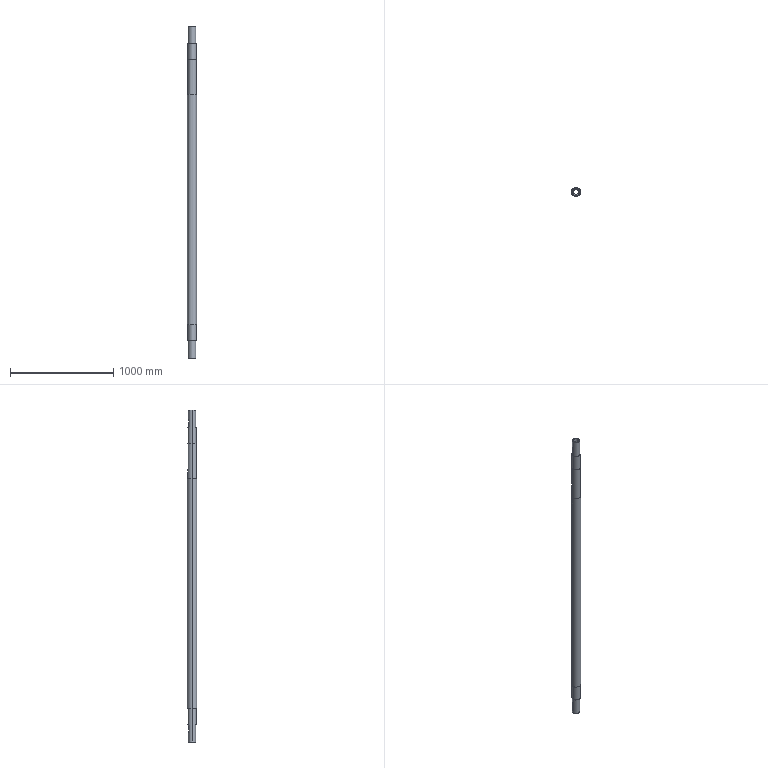Part | SolidWorks | features ICE 9, MirrorPattern 2, Chamfer 1, Extrusion 1 | 1 solid | 39 faces | box 89 x 89 x 3215 mm | volume 11535395 mm3 | cylinder 23 | plane 16 | commonest cylinder face diameters 20 x6 70 x4 80 x4 22 x3 53 x2 85 x2
STEP:
#1=CARTESIAN_POINT('',(0.,33.5,2636.));
#2=VERTEX_POINT('',#1);
#3=CARTESIAN_POINT('',(11.,33.5,2625.));
#4=VERTEX_POINT('',#3);
#5=CARTESIAN_POINT('',(0.,33.5,2625.));
#6=DIRECTION('',(0.,1.,0.));
#7=DIRECTION('',(0.,0.,1.));
#8=AXIS2_PLACEMENT_3D('',#5,#6,#7);
#9=CIRCLE('',#8,11.);
#10=EDGE_CURVE('',#2,#4,#9,.T.);
#11=ORIENTED_EDGE('',*,*,#10,.F.);
#12=CARTESIAN_POINT('',(0.,42.5,2636.));
#13=VERTEX_POINT('',#12);
#14=CARTESIAN_POINT('',(0.,33.5,2636.));
#15=DIRECTION('',(0.,1.,0.));
#16=VECTOR('',#15,1000.);
#17=LINE('',#14,#16);
#18=EDGE_CURVE('',#2,#13,#17,.T.);
#19=ORIENTED_EDGE('',*,*,#18,.T.);
#20=CARTESIAN_POINT('',(11.,41.052,2625.));
#21=VERTEX_POINT('',#20);
#22=CARTESIAN_POINT('',(0.,42.5,2636.));
#23=CARTESIAN_POINT('',(0.7204,42.5,2636.));
#24=CARTESIAN_POINT('',(1.452,42.481,2635.927));
#25=CARTESIAN_POINT('',(2.864,42.409,2635.645));
#26=CARTESIAN_POINT('',(3.551,42.357,2635.436));
#27=CARTESIAN_POINT('',(4.552,42.257,2635.02));
#28=CARTESIAN_POINT('',(4.881,42.22,2634.864));
#29=CARTESIAN_POINT('',(5.514,42.142,2634.525));
#30=CARTESIAN_POINT('',(5.821,42.101,2634.341));
#31=CARTESIAN_POINT('',(6.414,42.014,2633.943));
#32=CARTESIAN_POINT('',(6.701,41.969,2633.73));
#33=CARTESIAN_POINT('',(7.256,41.877,2633.276));
#34=CARTESIAN_POINT('',(7.524,41.829,2633.032));
#35=CARTESIAN_POINT('',(8.287,41.687,2632.269));
#36=CARTESIAN_POINT('',(8.74,41.594,2631.717));
#37=CARTESIAN_POINT('',(9.337,41.462,2630.827));
#38=CARTESIAN_POINT('',(9.522,41.42,2630.519));
#39=CARTESIAN_POINT('',(9.864,41.34,2629.882));
#40=CARTESIAN_POINT('',(10.019,41.302,2629.555));
#41=CARTESIAN_POINT('',(10.433,41.201,2628.56));
#42=CARTESIAN_POINT('',(10.642,41.146,2627.875));
#43=CARTESIAN_POINT('',(10.855,41.09,2626.814));
#44=CARTESIAN_POINT('',(10.91,41.076,2626.452));
#45=CARTESIAN_POINT('',(10.982,41.057,2625.728));
#46=CARTESIAN_POINT('',(11.,41.052,2625.365));
#47=CARTESIAN_POINT('',(11.,41.052,2625.));
#48=B_SPLINE_CURVE_WITH_KNOTS('',3,(#22,#23,#24,#25,#26,#27,#28,#29,#30,#31,#32,#33,#34,#35,#36,#37,#38,#39,#40,#41,#42,#43,#44,#45,#46,#47),.UNSPECIFIED.,.F.,.F.,(4,2,2,2,2,2,2,2,2,2,2,2,4),(0.01727,0.01943,0.02159,0.02267,0.02374,0.02482,0.0259,0.02806,0.02914,0.03021,0.03237,0.03345,0.03453),.UNSPECIFIED.);
#49=EDGE_CURVE('',#13,#21,#48,.T.);
#50=ORIENTED_EDGE('',*,*,#49,.T.);
#51=CARTESIAN_POINT('',(11.,33.5,2625.));
#52=DIRECTION('',(0.,1.,0.));
#53=VECTOR('',#52,1000.);
#54=LINE('',#51,#53);
#55=EDGE_CURVE('',#4,#21,#54,.T.);
#56=ORIENTED_EDGE('',*,*,#55,.F.);
#57=EDGE_LOOP('',(#11,#19,#50,#56));
#58=FACE_OUTER_BOUND('',#57,.T.);
#59=CARTESIAN_POINT('',(0.,33.5,2625.));
#60=DIRECTION('',(0.,1.,0.));
#61=DIRECTION('',(0.,0.,1.));
#62=AXIS2_PLACEMENT_3D('',#59,#60,#61);
#63=CYLINDRICAL_SURFACE('',#62,11.);
#64=ADVANCED_FACE('',(#58),#63,.F.);
#65=CARTESIAN_POINT('',(10.,27.5,150.));
#66=VERTEX_POINT('',#65);
#67=CARTESIAN_POINT('',(0.,27.5,160.));
#68=VERTEX_POINT('',#67);
#69=CARTESIAN_POINT('',(0.,27.5,150.));
#70=DIRECTION('',(0.,-1.,0.));
#71=DIRECTION('',(0.,0.,-1.));
#72=AXIS2_PLACEMENT_3D('',#69,#70,#71);
#73=CIRCLE('',#72,10.);
#74=EDGE_CURVE('',#66,#68,#73,.T.);
#75=ORIENTED_EDGE('',*,*,#74,.T.);
#76=CARTESIAN_POINT('',(0.,35.,160.));
#77=VERTEX_POINT('',#76);
#78=CARTESIAN_POINT('',(0.,27.5,160.));
#79=DIRECTION('',(0.,1.,0.));
#80=VECTOR('',#79,1000.);
#81=LINE('',#78,#80);
#82=EDGE_CURVE('',#68,#77,#81,.T.);
#83=ORIENTED_EDGE('',*,*,#82,.T.);
#84=CARTESIAN_POINT('',(10.,33.541,150.));
#85=VERTEX_POINT('',#84);
#86=CARTESIAN_POINT('',(0.,35.,160.));
#87=CARTESIAN_POINT('',(0.6556,35.,160.));
#88=CARTESIAN_POINT('',(1.322,34.981,159.934));
#89=CARTESIAN_POINT('',(2.606,34.909,159.677));
#90=CARTESIAN_POINT('',(3.23,34.856,159.487));
#91=CARTESIAN_POINT('',(4.141,34.756,159.108));
#92=CARTESIAN_POINT('',(4.439,34.719,158.966));
#93=CARTESIAN_POINT('',(5.015,34.64,158.658));
#94=CARTESIAN_POINT('',(5.293,34.598,158.49));
#95=CARTESIAN_POINT('',(5.833,34.512,158.129));
#96=CARTESIAN_POINT('',(6.093,34.466,157.936));
#97=CARTESIAN_POINT('',(6.597,34.374,157.522));
#98=CARTESIAN_POINT('',(6.841,34.326,157.301));
#99=CARTESIAN_POINT('',(7.534,34.183,156.608));
#100=CARTESIAN_POINT('',(7.945,34.088,156.108));
#101=CARTESIAN_POINT('',(8.668,33.912,155.029));
#102=CARTESIAN_POINT('',(8.982,33.829,154.444));
#103=CARTESIAN_POINT('',(9.483,33.692,153.24));
#104=CARTESIAN_POINT('',(9.674,33.637,152.617));
#105=CARTESIAN_POINT('',(9.868,33.58,151.65));
#106=CARTESIAN_POINT('',(9.918,33.565,151.321));
#107=CARTESIAN_POINT('',(9.984,33.546,150.663));
#108=CARTESIAN_POINT('',(10.,33.541,150.332));
#109=CARTESIAN_POINT('',(10.,33.541,150.));
#110=B_SPLINE_CURVE_WITH_KNOTS('',3,(#86,#87,#88,#89,#90,#91,#92,#93,#94,#95,#96,#97,#98,#99,#100,#101,#102,#103,#104,#105,#106,#107,#108,#109),.UNSPECIFIED.,.F.,.F.,(4,2,2,2,2,2,2,2,2,2,2,4),(0.01572,0.01768,0.01964,0.02062,0.02161,0.02259,0.02357,0.02553,0.02749,0.02946,0.03044,0.03142),.UNSPECIFIED.);
#111=EDGE_CURVE('',#77,#85,#110,.T.);
#112=ORIENTED_EDGE('',*,*,#111,.T.);
#113=CARTESIAN_POINT('',(10.,27.5,150.));
#114=DIRECTION('',(0.,1.,0.));
#115=VECTOR('',#114,1000.);
#116=LINE('',#113,#115);
#117=EDGE_CURVE('',#66,#85,#116,.T.);
#118=ORIENTED_EDGE('',*,*,#117,.F.);
#119=EDGE_LOOP('',(#75,#83,#112,#118));
#120=FACE_OUTER_BOUND('',#119,.T.);
#121=CARTESIAN_POINT('',(0.,27.5,150.));
#122=DIRECTION('',(0.,1.,0.));
#123=DIRECTION('',(0.,0.,1.));
#124=AXIS2_PLACEMENT_3D('',#121,#122,#123);
#125=CYLINDRICAL_SURFACE('',#124,10.);
#126=ADVANCED_FACE('',(#120),#125,.F.);
#127=CARTESIAN_POINT('',(0.,27.5,3130.));
#128=VERTEX_POINT('',#127);
#129=CARTESIAN_POINT('',(10.,27.5,3120.));
#130=VERTEX_POINT('',#129);
#131=CARTESIAN_POINT('',(0.,27.5,3120.));
#132=DIRECTION('',(0.,1.,0.));
#133=DIRECTION('',(0.,0.,1.));
#134=AXIS2_PLACEMENT_3D('',#131,#132,#133);
#135=CIRCLE('',#134,10.);
#136=EDGE_CURVE('',#128,#130,#135,.T.);
#137=ORIENTED_EDGE('',*,*,#136,.F.);
#138=CARTESIAN_POINT('',(0.,35.,3130.));
#139=VERTEX_POINT('',#138);
#140=CARTESIAN_POINT('',(0.,27.5,3130.));
#141=DIRECTION('',(0.,1.,0.));
#142=VECTOR('',#141,1000.);
#143=LINE('',#140,#142);
#144=EDGE_CURVE('',#128,#139,#143,.T.);
#145=ORIENTED_EDGE('',*,*,#144,.T.);
#146=CARTESIAN_POINT('',(10.,33.541,3120.));
#147=VERTEX_POINT('',#146);
#148=CARTESIAN_POINT('',(0.,35.,3130.));
#149=CARTESIAN_POINT('',(0.6556,35.,3130.));
#150=CARTESIAN_POINT('',(1.322,34.981,3129.934));
#151=CARTESIAN_POINT('',(2.606,34.909,3129.677));
#152=CARTESIAN_POINT('',(3.23,34.856,3129.487));
#153=CARTESIAN_POINT('',(4.141,34.756,3129.108));
#154=CARTESIAN_POINT('',(4.439,34.719,3128.966));
#155=CARTESIAN_POINT('',(5.015,34.64,3128.658));
#156=CARTESIAN_POINT('',(5.293,34.598,3128.49));
#157=CARTESIAN_POINT('',(5.833,34.512,3128.129));
#158=CARTESIAN_POINT('',(6.093,34.466,3127.936));
#159=CARTESIAN_POINT('',(6.597,34.374,3127.522));
#160=CARTESIAN_POINT('',(6.841,34.326,3127.301));
#161=CARTESIAN_POINT('',(7.534,34.183,3126.608));
#162=CARTESIAN_POINT('',(7.945,34.088,3126.108));
#163=CARTESIAN_POINT('',(8.668,33.912,3125.029));
#164=CARTESIAN_POINT('',(8.982,33.829,3124.444));
#165=CARTESIAN_POINT('',(9.483,33.692,3123.24));
#166=CARTESIAN_POINT('',(9.674,33.637,3122.617));
#167=CARTESIAN_POINT('',(9.868,33.58,3121.65));
#168=CARTESIAN_POINT('',(9.918,33.565,3121.321));
#169=CARTESIAN_POINT('',(9.984,33.546,3120.663));
#170=CARTESIAN_POINT('',(10.,33.541,3120.332));
#171=CARTESIAN_POINT('',(10.,33.541,3120.));
#172=B_SPLINE_CURVE_WITH_KNOTS('',3,(#148,#149,#150,#151,#152,#153,#154,#155,#156,#157,#158,#159,#160,#161,#162,#163,#164,#165,#166,#167,#168,#169,#170,#171),.UNSPECIFIED.,.F.,.F.,(4,2,2,2,2,2,2,2,2,2,2,4),(0.01572,0.01768,0.01964,0.02062,0.02161,0.02259,0.02357,0.02553,0.02749,0.02946,0.03044,0.03142),.UNSPECIFIED.);
#173=EDGE_CURVE('',#139,#147,#172,.T.);
#174=ORIENTED_EDGE('',*,*,#173,.T.);
#175=CARTESIAN_POINT('',(10.,27.5,3120.));
#176=DIRECTION('',(0.,1.,0.));
#177=VECTOR('',#176,1000.);
#178=LINE('',#175,#177);
#179=EDGE_CURVE('',#130,#147,#178,.T.);
#180=ORIENTED_EDGE('',*,*,#179,.F.);
#181=EDGE_LOOP('',(#137,#145,#174,#180));
#182=FACE_OUTER_BOUND('',#181,.T.);
#183=CARTESIAN_POINT('',(0.,27.5,3120.));
#184=DIRECTION('',(0.,1.,0.));
#185=DIRECTION('',(0.,0.,1.));
#186=AXIS2_PLACEMENT_3D('',#183,#184,#185);
#187=CYLINDRICAL_SURFACE('',#186,10.);
#188=ADVANCED_FACE('',(#182),#187,.F.);
#189=CARTESIAN_POINT('',(40.,0.,320.));
#190=VERTEX_POINT('',#189);
#191=CARTESIAN_POINT('',(-40.,0.,320.));
#192=VERTEX_POINT('',#191);
#193=CARTESIAN_POINT('',(0.,0.,320.));
#194=DIRECTION('',(0.,0.,1.));
#195=DIRECTION('',(1.,0.,0.));
#196=AXIS2_PLACEMENT_3D('',#193,#194,#195);
#197=CIRCLE('',#196,40.);
#198=EDGE_CURVE('',#190,#192,#197,.T.);
#199=ORIENTED_EDGE('',*,*,#198,.F.);
#200=CARTESIAN_POINT('',(40.,0.,165.));
#201=VERTEX_POINT('',#200);
#202=CARTESIAN_POINT('',(40.,0.,320.));
#203=DIRECTION('',(0.,0.,-1.));
#204=VECTOR('',#203,1000.);
#205=LINE('',#202,#204);
#206=EDGE_CURVE('',#190,#201,#205,.T.);
#207=ORIENTED_EDGE('',*,*,#206,.T.);
#208=CARTESIAN_POINT('',(-40.,0.,165.));
#209=VERTEX_POINT('',#208);
#210=CARTESIAN_POINT('',(0.,0.,165.));
#211=DIRECTION('',(0.,0.,1.));
#212=DIRECTION('',(1.,0.,0.));
#213=AXIS2_PLACEMENT_3D('',#210,#211,#212);
#214=CIRCLE('',#213,40.);
#215=EDGE_CURVE('',#201,#209,#214,.T.);
#216=ORIENTED_EDGE('',*,*,#215,.T.);
#217=CARTESIAN_POINT('',(-40.,0.,320.));
#218=DIRECTION('',(0.,0.,-1.));
#219=VECTOR('',#218,1000.);
#220=LINE('',#217,#219);
#221=EDGE_CURVE('',#192,#209,#220,.T.);
#222=ORIENTED_EDGE('',*,*,#221,.F.);
#223=EDGE_LOOP('',(#199,#207,#216,#222));
#224=FACE_OUTER_BOUND('',#223,.T.);
#225=CARTESIAN_POINT('',(0.,0.,320.));
#226=DIRECTION('',(0.,0.,-1.));
#227=DIRECTION('',(-1.,0.,0.));
#228=AXIS2_PLACEMENT_3D('',#225,#226,#227);
#229=CYLINDRICAL_SURFACE('',#228,40.);
#230=ADVANCED_FACE('',(#224),#229,.T.);
#231=CARTESIAN_POINT('',(-10.,33.541,3120.));
#232=VERTEX_POINT('',#231);
#233=CARTESIAN_POINT('',(-10.,33.541,3120.));
#234=CARTESIAN_POINT('',(-10.,33.541,3120.665));
#235=CARTESIAN_POINT('',(-9.934,33.561,3121.317));
#236=CARTESIAN_POINT('',(-9.742,33.617,3122.28));
#237=CARTESIAN_POINT('',(-9.662,33.64,3122.598));
#238=CARTESIAN_POINT('',(-9.47,33.695,3123.228));
#239=CARTESIAN_POINT('',(-9.358,33.726,3123.54));
#240=CARTESIAN_POINT('',(-8.981,33.829,3124.447));
#241=CARTESIAN_POINT('',(-8.673,33.91,3125.02));
#242=CARTESIAN_POINT('',(-8.129,34.044,3125.834));
#243=CARTESIAN_POINT('',(-7.932,34.09,3126.099));
#244=CARTESIAN_POINT('',(-7.516,34.184,3126.604));
#245=CARTESIAN_POINT('',(-7.298,34.232,3126.845));
#246=CARTESIAN_POINT('',(-6.609,34.374,3127.533));
#247=CARTESIAN_POINT('',(-6.108,34.467,3127.945));
#248=CARTESIAN_POINT('',(-5.015,34.643,3128.677));
#249=CARTESIAN_POINT('',(-4.438,34.723,3128.985));
#250=CARTESIAN_POINT('',(-3.536,34.822,3129.36));
#251=CARTESIAN_POINT('',(-3.229,34.852,3129.47));
#252=CARTESIAN_POINT('',(-2.6,34.905,3129.662));
#253=CARTESIAN_POINT('',(-2.278,34.927,3129.743));
#254=CARTESIAN_POINT('',(-1.308,34.982,3129.936));
#255=CARTESIAN_POINT('',(-0.6564,35.,3130.));
#256=CARTESIAN_POINT('',(0.,35.,3130.));
#257=B_SPLINE_CURVE_WITH_KNOTS('',3,(#233,#234,#235,#236,#237,#238,#239,#240,#241,#242,#243,#244,#245,#246,#247,#248,#249,#250,#251,#252,#253,#254,#255,#256),.UNSPECIFIED.,.F.,.F.,(4,2,2,2,2,2,2,2,2,2,2,4),(0.,0.001965,0.002947,0.00393,0.005894,0.006877,0.007859,0.009824,0.01179,0.01277,0.01375,0.01572),.UNSPECIFIED.);
#258=EDGE_CURVE('',#232,#139,#257,.T.);
#259=ORIENTED_EDGE('',*,*,#258,.F.);
#260=CARTESIAN_POINT('',(-10.,33.541,3065.));
#261=VERTEX_POINT('',#260);
#262=CARTESIAN_POINT('',(-10.,33.541,2943.934));
#263=DIRECTION('',(0.,0.,1.));
#264=VECTOR('',#263,1000.);
#265=LINE('',#262,#264);
#266=EDGE_CURVE('',#261,#232,#265,.T.);
#267=ORIENTED_EDGE('',*,*,#266,.F.);
#268=CARTESIAN_POINT('',(10.,33.541,3065.));
#269=VERTEX_POINT('',#268);
#270=CARTESIAN_POINT('',(10.,33.541,3065.));
#271=CARTESIAN_POINT('',(10.,33.541,3064.336));
#272=CARTESIAN_POINT('',(9.934,33.561,3063.683));
#273=CARTESIAN_POINT('',(9.742,33.617,3062.722));
#274=CARTESIAN_POINT('',(9.663,33.64,3062.404));
#275=CARTESIAN_POINT('',(9.471,33.694,3061.774));
#276=CARTESIAN_POINT('',(9.359,33.726,3061.462));
#277=CARTESIAN_POINT('',(8.982,33.829,3060.555));
#278=CARTESIAN_POINT('',(8.675,33.91,3059.982));
#279=CARTESIAN_POINT('',(8.131,34.043,3059.169));
#280=CARTESIAN_POINT('',(7.934,34.089,3058.905));
#281=CARTESIAN_POINT('',(7.519,34.183,3058.399));
#282=CARTESIAN_POINT('',(7.301,34.231,3058.159));
#283=CARTESIAN_POINT('',(6.613,34.373,3057.471));
#284=CARTESIAN_POINT('',(6.112,34.467,3057.058));
#285=CARTESIAN_POINT('',(5.02,34.642,3056.327));
#286=CARTESIAN_POINT('',(4.444,34.722,3056.018));
#287=CARTESIAN_POINT('',(3.543,34.822,3055.643));
#288=CARTESIAN_POINT('',(3.236,34.852,3055.532));
#289=CARTESIAN_POINT('',(2.608,34.904,3055.341));
#290=CARTESIAN_POINT('',(2.286,34.927,3055.259));
#291=CARTESIAN_POINT('',(1.317,34.981,3055.065));
#292=CARTESIAN_POINT('',(0.6655,35.,3055.001));
#293=CARTESIAN_POINT('',(-0.6464,35.,3054.999));
#294=CARTESIAN_POINT('',(-1.313,34.981,3055.065));
#295=CARTESIAN_POINT('',(-2.598,34.909,3055.321));
#296=CARTESIAN_POINT('',(-3.223,34.857,3055.511));
#297=CARTESIAN_POINT('',(-4.135,34.756,3055.889));
#298=CARTESIAN_POINT('',(-4.433,34.719,3056.031));
#299=CARTESIAN_POINT('',(-5.009,34.641,3056.339));
#300=CARTESIAN_POINT('',(-5.288,34.599,3056.506));
#301=CARTESIAN_POINT('',(-5.828,34.512,3056.867));
#302=CARTESIAN_POINT('',(-6.089,34.467,3057.061));
#303=CARTESIAN_POINT('',(-6.593,34.374,3057.474));
#304=CARTESIAN_POINT('',(-6.838,34.326,3057.696));
#305=CARTESIAN_POINT('',(-7.531,34.183,3058.388));
#306=CARTESIAN_POINT('',(-7.942,34.089,3058.889));
#307=CARTESIAN_POINT('',(-8.666,33.912,3059.969));
#308=CARTESIAN_POINT('',(-8.981,33.829,3060.554));
#309=CARTESIAN_POINT('',(-9.483,33.692,3061.759));
#310=CARTESIAN_POINT('',(-9.674,33.637,3062.382));
#311=CARTESIAN_POINT('',(-9.868,33.58,3063.349));
#312=CARTESIAN_POINT('',(-9.918,33.565,3063.678));
#313=CARTESIAN_POINT('',(-9.983,33.546,3064.337));
#314=CARTESIAN_POINT('',(-10.,33.541,3064.668));
#315=CARTESIAN_POINT('',(-10.,33.541,3065.));
#316=B_SPLINE_CURVE_WITH_KNOTS('',3,(#270,#271,#272,#273,#274,#275,#276,#277,#278,#279,#280,#281,#282,#283,#284,#285,#286,#287,#288,#289,#290,#291,#292,#293,#294,#295,#296,#297,#298,#299,#300,#301,#302,#303,#304,#305,#306,#307,#308,#309,#310,#311,#312,#313,#314,#315),.UNSPECIFIED.,.F.,.F.,(4,2,2,2,2,2,2,2,2,2,2,2,2,2,2,2,2,2,2,2,2,2,4),(0.,0.001964,0.002945,0.003927,0.005891,0.006873,0.007855,0.009818,0.01178,0.01276,0.01375,0.01571,0.01767,0.01964,0.02062,0.0216,0.02258,0.02356,0.02553,0.02749,0.02945,0.03044,0.03142),.UNSPECIFIED.);
#317=EDGE_CURVE('',#269,#261,#316,.T.);
#318=ORIENTED_EDGE('',*,*,#317,.F.);
#319=CARTESIAN_POINT('',(10.,33.541,2943.934));
#320=DIRECTION('',(0.,0.,-1.));
#321=VECTOR('',#320,1000.);
#322=LINE('',#319,#321);
#323=EDGE_CURVE('',#147,#269,#322,.T.);
#324=ORIENTED_EDGE('',*,*,#323,.F.);
#325=ORIENTED_EDGE('',*,*,#173,.F.);
#326=EDGE_LOOP('',(#259,#267,#318,#324,#325));
#327=FACE_BOUND('',#326,.T.);
#328=CARTESIAN_POINT('',(-35.,0.,3050.));
#329=VERTEX_POINT('',#328);
#330=CARTESIAN_POINT('',(35.,0.,3050.));
#331=VERTEX_POINT('',#330);
#332=CARTESIAN_POINT('',(0.,0.,3050.));
#333=DIRECTION('',(0.,0.,-1.));
#334=DIRECTION('',(1.,0.,0.));
#335=AXIS2_PLACEMENT_3D('',#332,#333,#334);
#336=CIRCLE('',#335,35.);
#337=EDGE_CURVE('',#329,#331,#336,.T.);
#338=ORIENTED_EDGE('',*,*,#337,.F.);
#339=CARTESIAN_POINT('',(-35.,0.,3215.));
#340=VERTEX_POINT('',#339);
#341=CARTESIAN_POINT('',(-35.,0.,2943.934));
#342=DIRECTION('',(0.,0.,1.));
#343=VECTOR('',#342,1000.);
#344=LINE('',#341,#343);
#345=EDGE_CURVE('',#329,#340,#344,.T.);
#346=ORIENTED_EDGE('',*,*,#345,.T.);
#347=CARTESIAN_POINT('',(35.,0.,3215.));
#348=VERTEX_POINT('',#347);
#349=CARTESIAN_POINT('',(0.,0.,3215.));
#350=DIRECTION('',(0.,0.,1.));
#351=DIRECTION('',(1.,0.,0.));
#352=AXIS2_PLACEMENT_3D('',#349,#350,#351);
#353=CIRCLE('',#352,35.);
#354=EDGE_CURVE('',#348,#340,#353,.T.);
#355=ORIENTED_EDGE('',*,*,#354,.F.);
#356=CARTESIAN_POINT('',(35.,0.,2943.934));
#357=DIRECTION('',(0.,0.,1.));
#358=VECTOR('',#357,1000.);
#359=LINE('',#356,#358);
#360=EDGE_CURVE('',#331,#348,#359,.T.);
#361=ORIENTED_EDGE('',*,*,#360,.F.);
#362=EDGE_LOOP('',(#338,#346,#355,#361));
#363=FACE_OUTER_BOUND('',#362,.T.);
#364=CARTESIAN_POINT('',(0.,0.,2943.934));
#365=DIRECTION('',(0.,0.,1.));
#366=DIRECTION('',(1.,0.,0.));
#367=AXIS2_PLACEMENT_3D('',#364,#365,#366);
#368=CYLINDRICAL_SURFACE('',#367,35.);
#369=ADVANCED_FACE('',(#327,#363),#368,.T.);
#370=CARTESIAN_POINT('',(-26.5,0.,0.));
#371=VERTEX_POINT('',#370);
#372=CARTESIAN_POINT('',(26.5,0.,0.));
#373=VERTEX_POINT('',#372);
#374=CARTESIAN_POINT('',(0.,0.,0.));
#375=DIRECTION('',(0.,0.,1.));
#376=DIRECTION('',(1.,0.,0.));
#377=AXIS2_PLACEMENT_3D('',#374,#375,#376);
#378=CIRCLE('',#377,26.5);
#379=EDGE_CURVE('',#371,#373,#378,.T.);
#380=ORIENTED_EDGE('',*,*,#379,.F.);
#381=CARTESIAN_POINT('',(-26.5,0.,3215.));
#382=VERTEX_POINT('',#381);
#383=CARTESIAN_POINT('',(-26.5,0.,0.));
#384=DIRECTION('',(0.,0.,1.));
#385=VECTOR('',#384,1000.);
#386=LINE('',#383,#385);
#387=EDGE_CURVE('',#371,#382,#386,.T.);
#388=ORIENTED_EDGE('',*,*,#387,.T.);
#389=CARTESIAN_POINT('',(26.5,0.,3215.));
#390=VERTEX_POINT('',#389);
#391=CARTESIAN_POINT('',(0.,0.,3215.));
#392=DIRECTION('',(0.,0.,1.));
#393=DIRECTION('',(1.,0.,0.));
#394=AXIS2_PLACEMENT_3D('',#391,#392,#393);
#395=CIRCLE('',#394,26.5);
#396=EDGE_CURVE('',#382,#390,#395,.T.);
#397=ORIENTED_EDGE('',*,*,#396,.T.);
#398=CARTESIAN_POINT('',(26.5,0.,0.));
#399=DIRECTION('',(0.,0.,1.));
#400=VECTOR('',#399,1000.);
#401=LINE('',#398,#400);
#402=EDGE_CURVE('',#373,#390,#401,.T.);
#403=ORIENTED_EDGE('',*,*,#402,.F.);
#404=EDGE_LOOP('',(#380,#388,#397,#403));
#405=FACE_OUTER_BOUND('',#404,.T.);
#406=CARTESIAN_POINT('',(0.,0.,0.));
#407=DIRECTION('',(0.,0.,1.));
#408=DIRECTION('',(1.,0.,0.));
#409=AXIS2_PLACEMENT_3D('',#406,#407,#408);
#410=CYLINDRICAL_SURFACE('',#409,26.5);
#411=ADVANCED_FACE('',(#405),#410,.F.);
#412=CARTESIAN_POINT('',(40.,0.,2895.));
#413=VERTEX_POINT('',#412);
#414=CARTESIAN_POINT('',(-40.,0.,2895.));
#415=VERTEX_POINT('',#414);
#416=CARTESIAN_POINT('',(0.,0.,2895.));
#417=DIRECTION('',(0.,0.,1.));
#418=DIRECTION('',(1.,0.,0.));
#419=AXIS2_PLACEMENT_3D('',#416,#417,#418);
#420=CIRCLE('',#419,40.);
#421=EDGE_CURVE('',#413,#415,#420,.T.);
#422=ORIENTED_EDGE('',*,*,#421,.T.);
#423=CARTESIAN_POINT('',(-40.,0.,3050.));
#424=VERTEX_POINT('',#423);
#425=CARTESIAN_POINT('',(-40.,0.,2895.));
#426=DIRECTION('',(0.,0.,1.));
#427=VECTOR('',#426,1000.);
#428=LINE('',#425,#427);
#429=EDGE_CURVE('',#415,#424,#428,.T.);
#430=ORIENTED_EDGE('',*,*,#429,.T.);
#431=CARTESIAN_POINT('',(40.,0.,3050.));
#432=VERTEX_POINT('',#431);
#433=CARTESIAN_POINT('',(0.,0.,3050.));
#434=DIRECTION('',(0.,0.,1.));
#435=DIRECTION('',(1.,0.,0.));
#436=AXIS2_PLACEMENT_3D('',#433,#434,#435);
#437=CIRCLE('',#436,40.);
#438=EDGE_CURVE('',#432,#424,#437,.T.);
#439=ORIENTED_EDGE('',*,*,#438,.F.);
#440=CARTESIAN_POINT('',(40.,0.,2895.));
#441=DIRECTION('',(0.,0.,1.));
#442=VECTOR('',#441,1000.);
#443=LINE('',#440,#442);
#444=EDGE_CURVE('',#413,#432,#443,.T.);
#445=ORIENTED_EDGE('',*,*,#444,.F.);
#446=EDGE_LOOP('',(#422,#430,#439,#445));
#447=FACE_OUTER_BOUND('',#446,.T.);
#448=CARTESIAN_POINT('',(0.,0.,2895.));
#449=DIRECTION('',(0.,0.,1.));
#450=DIRECTION('',(1.,0.,0.));
#451=AXIS2_PLACEMENT_3D('',#448,#449,#450);
#452=CYLINDRICAL_SURFACE('',#451,40.);
#453=ADVANCED_FACE('',(#447),#452,.T.);
#454=CARTESIAN_POINT('',(44.5,0.,2555.));
#455=VERTEX_POINT('',#454);
#456=CARTESIAN_POINT('',(-44.5,0.,2555.));
#457=VERTEX_POINT('',#456);
#458=CARTESIAN_POINT('',(0.,0.,2555.));
#459=DIRECTION('',(0.,0.,1.));
#460=DIRECTION('',(1.,0.,0.));
#461=AXIS2_PLACEMENT_3D('',#458,#459,#460);
#462=CIRCLE('',#461,44.5);
#463=EDGE_CURVE('',#455,#457,#462,.T.);
#464=ORIENTED_EDGE('',*,*,#463,.F.);
#465=CARTESIAN_POINT('',(44.5,0.,320.));
#466=VERTEX_POINT('',#465);
#467=CARTESIAN_POINT('',(44.5,0.,3215.));
#468=DIRECTION('',(0.,0.,-1.));
#469=VECTOR('',#468,1000.);
#470=LINE('',#467,#469);
#471=EDGE_CURVE('',#455,#466,#470,.T.);
#472=ORIENTED_EDGE('',*,*,#471,.T.);
#473=CARTESIAN_POINT('',(-44.5,0.,320.));
#474=VERTEX_POINT('',#473);
#475=CARTESIAN_POINT('',(0.,0.,320.));
#476=DIRECTION('',(0.,0.,1.));
#477=DIRECTION('',(1.,0.,0.));
#478=AXIS2_PLACEMENT_3D('',#475,#476,#477);
#479=CIRCLE('',#478,44.5);
#480=EDGE_CURVE('',#466,#474,#479,.T.);
#481=ORIENTED_EDGE('',*,*,#480,.T.);
#482=CARTESIAN_POINT('',(-44.5,0.,3215.));
#483=DIRECTION('',(0.,0.,-1.));
#484=VECTOR('',#483,1000.);
#485=LINE('',#482,#484);
#486=EDGE_CURVE('',#457,#474,#485,.T.);
#487=ORIENTED_EDGE('',*,*,#486,.F.);
#488=EDGE_LOOP('',(#464,#472,#481,#487));
#489=FACE_OUTER_BOUND('',#488,.T.);
#490=CARTESIAN_POINT('',(0.,0.,3215.));
#491=DIRECTION('',(0.,0.,-1.));
#492=DIRECTION('',(-1.,0.,0.));
#493=AXIS2_PLACEMENT_3D('',#490,#491,#492);
#494=CYLINDRICAL_SURFACE('',#493,44.5);
#495=ADVANCED_FACE('',(#489),#494,.T.);
#496=CARTESIAN_POINT('',(10.,33.541,95.));
#497=VERTEX_POINT('',#496);
#498=CARTESIAN_POINT('',(-10.,33.541,95.));
#499=VERTEX_POINT('',#498);
#500=CARTESIAN_POINT('',(10.,33.541,95.));
#501=CARTESIAN_POINT('',(10.,33.541,94.336));
#502=CARTESIAN_POINT('',(9.934,33.561,93.683));
#503=CARTESIAN_POINT('',(9.742,33.617,92.722));
#504=CARTESIAN_POINT('',(9.663,33.64,92.404));
#505=CARTESIAN_POINT('',(9.471,33.694,91.774));
#506=CARTESIAN_POINT('',(9.359,33.726,91.462));
#507=CARTESIAN_POINT('',(8.982,33.829,90.555));
#508=CARTESIAN_POINT('',(8.675,33.91,89.982));
#509=CARTESIAN_POINT('',(8.131,34.043,89.169));
#510=CARTESIAN_POINT('',(7.934,34.089,88.905));
#511=CARTESIAN_POINT('',(7.519,34.183,88.399));
#512=CARTESIAN_POINT('',(7.301,34.231,88.159));
#513=CARTESIAN_POINT('',(6.613,34.373,87.471));
#514=CARTESIAN_POINT('',(6.112,34.467,87.058));
#515=CARTESIAN_POINT('',(5.02,34.642,86.327));
#516=CARTESIAN_POINT('',(4.444,34.722,86.018));
#517=CARTESIAN_POINT('',(3.543,34.822,85.643));
#518=CARTESIAN_POINT('',(3.236,34.852,85.532));
#519=CARTESIAN_POINT('',(2.608,34.904,85.341));
#520=CARTESIAN_POINT('',(2.286,34.927,85.259));
#521=CARTESIAN_POINT('',(1.317,34.981,85.065));
#522=CARTESIAN_POINT('',(0.6655,35.,85.001));
#523=CARTESIAN_POINT('',(-0.6464,35.,84.999));
#524=CARTESIAN_POINT('',(-1.313,34.981,85.065));
#525=CARTESIAN_POINT('',(-2.598,34.909,85.321));
#526=CARTESIAN_POINT('',(-3.223,34.857,85.511));
#527=CARTESIAN_POINT('',(-4.135,34.756,85.889));
#528=CARTESIAN_POINT('',(-4.433,34.719,86.031));
#529=CARTESIAN_POINT('',(-5.009,34.641,86.339));
#530=CARTESIAN_POINT('',(-5.288,34.599,86.506));
#531=CARTESIAN_POINT('',(-5.828,34.512,86.867));
#532=CARTESIAN_POINT('',(-6.089,34.467,87.061));
#533=CARTESIAN_POINT('',(-6.593,34.374,87.474));
#534=CARTESIAN_POINT('',(-6.838,34.326,87.696));
#535=CARTESIAN_POINT('',(-7.531,34.183,88.388));
#536=CARTESIAN_POINT('',(-7.942,34.089,88.889));
#537=CARTESIAN_POINT('',(-8.666,33.912,89.969));
#538=CARTESIAN_POINT('',(-8.981,33.829,90.554));
#539=CARTESIAN_POINT('',(-9.483,33.692,91.759));
#540=CARTESIAN_POINT('',(-9.674,33.637,92.382));
#541=CARTESIAN_POINT('',(-9.868,33.58,93.349));
#542=CARTESIAN_POINT('',(-9.918,33.565,93.678));
#543=CARTESIAN_POINT('',(-9.983,33.546,94.337));
#544=CARTESIAN_POINT('',(-10.,33.541,94.668));
#545=CARTESIAN_POINT('',(-10.,33.541,95.));
#546=B_SPLINE_CURVE_WITH_KNOTS('',3,(#500,#501,#502,#503,#504,#505,#506,#507,#508,#509,#510,#511,#512,#513,#514,#515,#516,#517,#518,#519,#520,#521,#522,#523,#524,#525,#526,#527,#528,#529,#530,#531,#532,#533,#534,#535,#536,#537,#538,#539,#540,#541,#542,#543,#544,#545),.UNSPECIFIED.,.F.,.F.,(4,2,2,2,2,2,2,2,2,2,2,2,2,2,2,2,2,2,2,2,2,2,4),(0.,0.001964,0.002945,0.003927,0.005891,0.006873,0.007855,0.009818,0.01178,0.01276,0.01375,0.01571,0.01767,0.01964,0.02062,0.0216,0.02258,0.02356,0.02553,0.02749,0.02945,0.03044,0.03142),.UNSPECIFIED.);
#547=EDGE_CURVE('',#497,#499,#546,.T.);
#548=ORIENTED_EDGE('',*,*,#547,.F.);
#549=CARTESIAN_POINT('',(10.,33.541,3156.066));
#550=DIRECTION('',(0.,0.,-1.));
#551=VECTOR('',#550,1000.);
#552=LINE('',#549,#551);
#553=EDGE_CURVE('',#85,#497,#552,.T.);
#554=ORIENTED_EDGE('',*,*,#553,.F.);
#555=ORIENTED_EDGE('',*,*,#111,.F.);
#556=CARTESIAN_POINT('',(-10.,33.541,150.));
#557=VERTEX_POINT('',#556);
#558=CARTESIAN_POINT('',(-10.,33.541,150.));
#559=CARTESIAN_POINT('',(-10.,33.541,150.665));
#560=CARTESIAN_POINT('',(-9.934,33.561,151.317));
#561=CARTESIAN_POINT('',(-9.742,33.617,152.28));
#562=CARTESIAN_POINT('',(-9.662,33.64,152.598));
#563=CARTESIAN_POINT('',(-9.47,33.695,153.228));
#564=CARTESIAN_POINT('',(-9.358,33.726,153.54));
#565=CARTESIAN_POINT('',(-8.981,33.829,154.447));
#566=CARTESIAN_POINT('',(-8.673,33.91,155.02));
#567=CARTESIAN_POINT('',(-8.129,34.044,155.834));
#568=CARTESIAN_POINT('',(-7.932,34.09,156.099));
#569=CARTESIAN_POINT('',(-7.516,34.184,156.604));
#570=CARTESIAN_POINT('',(-7.298,34.232,156.845));
#571=CARTESIAN_POINT('',(-6.609,34.374,157.533));
#572=CARTESIAN_POINT('',(-6.108,34.467,157.945));
#573=CARTESIAN_POINT('',(-5.015,34.643,158.677));
#574=CARTESIAN_POINT('',(-4.438,34.723,158.985));
#575=CARTESIAN_POINT('',(-3.536,34.822,159.36));
#576=CARTESIAN_POINT('',(-3.229,34.852,159.47));
#577=CARTESIAN_POINT('',(-2.6,34.905,159.662));
#578=CARTESIAN_POINT('',(-2.278,34.927,159.743));
#579=CARTESIAN_POINT('',(-1.308,34.982,159.936));
#580=CARTESIAN_POINT('',(-0.6564,35.,160.));
#581=CARTESIAN_POINT('',(0.,35.,160.));
#582=B_SPLINE_CURVE_WITH_KNOTS('',3,(#558,#559,#560,#561,#562,#563,#564,#565,#566,#567,#568,#569,#570,#571,#572,#573,#574,#575,#576,#577,#578,#579,#580,#581),.UNSPECIFIED.,.F.,.F.,(4,2,2,2,2,2,2,2,2,2,2,4),(0.,0.001965,0.002947,0.00393,0.005894,0.006877,0.007859,0.009824,0.01179,0.01277,0.01375,0.01572),.UNSPECIFIED.);
#583=EDGE_CURVE('',#557,#77,#582,.T.);
#584=ORIENTED_EDGE('',*,*,#583,.F.);
#585=CARTESIAN_POINT('',(-10.,33.541,3156.066));
#586=DIRECTION('',(0.,0.,1.));
#587=VECTOR('',#586,1000.);
#588=LINE('',#585,#587);
#589=EDGE_CURVE('',#499,#557,#588,.T.);
#590=ORIENTED_EDGE('',*,*,#589,.F.);
#591=EDGE_LOOP('',(#548,#554,#555,#584,#590));
#592=FACE_BOUND('',#591,.T.);
#593=CARTESIAN_POINT('',(-35.,0.,165.));
#594=VERTEX_POINT('',#593);
#595=CARTESIAN_POINT('',(35.,0.,165.));
#596=VERTEX_POINT('',#595);
#597=CARTESIAN_POINT('',(0.,0.,165.));
#598=DIRECTION('',(0.,0.,-1.));
#599=DIRECTION('',(-1.,0.,0.));
#600=AXIS2_PLACEMENT_3D('',#597,#598,#599);
#601=CIRCLE('',#600,35.);
#602=EDGE_CURVE('',#594,#596,#601,.T.);
#603=ORIENTED_EDGE('',*,*,#602,.T.);
#604=CARTESIAN_POINT('',(35.,0.,0.));
#605=VERTEX_POINT('',#604);
#606=CARTESIAN_POINT('',(35.,0.,3156.066));
#607=DIRECTION('',(0.,0.,-1.));
#608=VECTOR('',#607,1000.);
#609=LINE('',#606,#608);
#610=EDGE_CURVE('',#596,#605,#609,.T.);
#611=ORIENTED_EDGE('',*,*,#610,.T.);
#612=CARTESIAN_POINT('',(-35.,0.,0.));
#613=VERTEX_POINT('',#612);
#614=CARTESIAN_POINT('',(0.,0.,0.));
#615=DIRECTION('',(0.,0.,1.));
#616=DIRECTION('',(1.,0.,0.));
#617=AXIS2_PLACEMENT_3D('',#614,#615,#616);
#618=CIRCLE('',#617,35.);
#619=EDGE_CURVE('',#605,#613,#618,.T.);
#620=ORIENTED_EDGE('',*,*,#619,.T.);
#621=CARTESIAN_POINT('',(-35.,0.,3156.066));
#622=DIRECTION('',(0.,0.,-1.));
#623=VECTOR('',#622,1000.);
#624=LINE('',#621,#623);
#625=EDGE_CURVE('',#594,#613,#624,.T.);
#626=ORIENTED_EDGE('',*,*,#625,.F.);
#627=EDGE_LOOP('',(#603,#611,#620,#626));
#628=FACE_OUTER_BOUND('',#627,.T.);
#629=CARTESIAN_POINT('',(0.,0.,3156.066));
#630=DIRECTION('',(0.,0.,-1.));
#631=DIRECTION('',(-1.,0.,0.));
#632=AXIS2_PLACEMENT_3D('',#629,#630,#631);
#633=CYLINDRICAL_SURFACE('',#632,35.);
#634=ADVANCED_FACE('',(#592,#628),#633,.T.);
#635=CARTESIAN_POINT('',(-11.,41.052,2625.));
#636=VERTEX_POINT('',#635);
#637=CARTESIAN_POINT('',(-11.,41.052,2625.));
#638=CARTESIAN_POINT('',(-11.,41.052,2625.73));
#639=CARTESIAN_POINT('',(-10.928,41.071,2626.448));
#640=CARTESIAN_POINT('',(-10.717,41.127,2627.506));
#641=CARTESIAN_POINT('',(-10.629,41.15,2627.855));
#642=CARTESIAN_POINT('',(-10.418,41.203,2628.548));
#643=CARTESIAN_POINT('',(-10.295,41.235,2628.892));
#644=CARTESIAN_POINT('',(-9.88,41.337,2629.89));
#645=CARTESIAN_POINT('',(-9.541,41.417,2630.52));
#646=CARTESIAN_POINT('',(-8.943,41.549,2631.416));
#647=CARTESIAN_POINT('',(-8.726,41.595,2631.707));
#648=CARTESIAN_POINT('',(-8.268,41.689,2632.264));
#649=CARTESIAN_POINT('',(-8.028,41.736,2632.529));
#650=CARTESIAN_POINT('',(-7.269,41.877,2633.286));
#651=CARTESIAN_POINT('',(-6.717,41.97,2633.741));
#652=CARTESIAN_POINT('',(-5.816,42.101,2634.344));
#653=CARTESIAN_POINT('',(-5.505,42.143,2634.53));
#654=CARTESIAN_POINT('',(-4.872,42.221,2634.869));
#655=CARTESIAN_POINT('',(-4.549,42.257,2635.022));
#656=CARTESIAN_POINT('',(-3.887,42.323,2635.297));
#657=CARTESIAN_POINT('',(-3.549,42.353,2635.418));
#658=CARTESIAN_POINT('',(-2.859,42.405,2635.628));
#659=CARTESIAN_POINT('',(-2.504,42.428,2635.717));
#660=CARTESIAN_POINT('',(-1.437,42.482,2635.93));
#661=CARTESIAN_POINT('',(-0.7212,42.5,2636.));
#662=CARTESIAN_POINT('',(0.,42.5,2636.));
#663=B_SPLINE_CURVE_WITH_KNOTS('',3,(#637,#638,#639,#640,#641,#642,#643,#644,#645,#646,#647,#648,#649,#650,#651,#652,#653,#654,#655,#656,#657,#658,#659,#660,#661,#662),.UNSPECIFIED.,.F.,.F.,(4,2,2,2,2,2,2,2,2,2,2,2,4),(0.,0.002159,0.003239,0.004318,0.006478,0.007557,0.008637,0.0108,0.01188,0.01296,0.01403,0.01511,0.01727),.UNSPECIFIED.);
#664=EDGE_CURVE('',#636,#13,#663,.T.);
#665=ORIENTED_EDGE('',*,*,#664,.F.);
#666=CARTESIAN_POINT('',(-11.,41.052,2570.));
#667=VERTEX_POINT('',#666);
#668=CARTESIAN_POINT('',(-11.,41.052,2555.));
#669=DIRECTION('',(0.,0.,1.));
#670=VECTOR('',#669,1000.);
#671=LINE('',#668,#670);
#672=EDGE_CURVE('',#667,#636,#671,.T.);
#673=ORIENTED_EDGE('',*,*,#672,.F.);
#674=CARTESIAN_POINT('',(11.,41.052,2570.));
#675=VERTEX_POINT('',#674);
#676=CARTESIAN_POINT('',(-11.,41.052,2570.));
#677=CARTESIAN_POINT('',(-11.,41.052,2569.27));
#678=CARTESIAN_POINT('',(-10.928,41.071,2568.553));
#679=CARTESIAN_POINT('',(-10.717,41.127,2567.496));
#680=CARTESIAN_POINT('',(-10.63,41.149,2567.146));
#681=CARTESIAN_POINT('',(-10.419,41.203,2566.454));
#682=CARTESIAN_POINT('',(-10.296,41.234,2566.111));
#683=CARTESIAN_POINT('',(-9.881,41.336,2565.113));
#684=CARTESIAN_POINT('',(-9.543,41.417,2564.482));
#685=CARTESIAN_POINT('',(-8.945,41.549,2563.588));
#686=CARTESIAN_POINT('',(-8.729,41.595,2563.296));
#687=CARTESIAN_POINT('',(-8.271,41.688,2562.74));
#688=CARTESIAN_POINT('',(-8.031,41.735,2562.474));
#689=CARTESIAN_POINT('',(-7.273,41.876,2561.717));
#690=CARTESIAN_POINT('',(-6.722,41.969,2561.263));
#691=CARTESIAN_POINT('',(-5.821,42.101,2560.66));
#692=CARTESIAN_POINT('',(-5.511,42.142,2560.473));
#693=CARTESIAN_POINT('',(-4.879,42.22,2560.135));
#694=CARTESIAN_POINT('',(-4.555,42.256,2559.981));
#695=CARTESIAN_POINT('',(-3.894,42.323,2559.706));
#696=CARTESIAN_POINT('',(-3.557,42.352,2559.585));
#697=CARTESIAN_POINT('',(-2.867,42.405,2559.374));
#698=CARTESIAN_POINT('',(-2.512,42.427,2559.285));
#699=CARTESIAN_POINT('',(-1.446,42.481,2559.071));
#700=CARTESIAN_POINT('',(-0.7307,42.5,2559.001));
#701=CARTESIAN_POINT('',(0.7108,42.5,2558.999));
#702=CARTESIAN_POINT('',(1.443,42.481,2559.071));
#703=CARTESIAN_POINT('',(2.856,42.41,2559.353));
#704=CARTESIAN_POINT('',(3.544,42.357,2559.561));
#705=CARTESIAN_POINT('',(4.545,42.258,2559.976));
#706=CARTESIAN_POINT('',(4.874,42.221,2560.132));
#707=CARTESIAN_POINT('',(5.508,42.143,2560.472));
#708=CARTESIAN_POINT('',(5.815,42.101,2560.656));
#709=CARTESIAN_POINT('',(6.41,42.015,2561.053));
#710=CARTESIAN_POINT('',(6.697,41.97,2561.266));
#711=CARTESIAN_POINT('',(7.252,41.878,2561.721));
#712=CARTESIAN_POINT('',(7.52,41.83,2561.964));
#713=CARTESIAN_POINT('',(8.284,41.688,2562.728));
#714=CARTESIAN_POINT('',(8.737,41.594,2563.279));
#715=CARTESIAN_POINT('',(9.335,41.463,2564.17));
#716=CARTESIAN_POINT('',(9.52,41.42,2564.478));
#717=CARTESIAN_POINT('',(9.863,41.34,2565.115));
#718=CARTESIAN_POINT('',(10.018,41.303,2565.443));
#719=CARTESIAN_POINT('',(10.432,41.201,2566.438));
#720=CARTESIAN_POINT('',(10.642,41.146,2567.123));
#721=CARTESIAN_POINT('',(10.855,41.09,2568.185));
#722=CARTESIAN_POINT('',(10.91,41.076,2568.547));
#723=CARTESIAN_POINT('',(10.982,41.057,2569.271));
#724=CARTESIAN_POINT('',(11.,41.052,2569.635));
#725=CARTESIAN_POINT('',(11.,41.052,2570.));
#726=B_SPLINE_CURVE_WITH_KNOTS('',3,(#676,#677,#678,#679,#680,#681,#682,#683,#684,#685,#686,#687,#688,#689,#690,#691,#692,#693,#694,#695,#696,#697,#698,#699,#700,#701,#702,#703,#704,#705,#706,#707,#708,#709,#710,#711,#712,#713,#714,#715,#716,#717,#718,#719,#720,#721,#722,#723,#724,#725),.UNSPECIFIED.,.F.,.F.,(4,2,2,2,2,2,2,2,2,2,2,2,2,2,2,2,2,2,2,2,2,2,2,2,4),(0.,0.002158,0.003237,0.004316,0.006474,0.007553,0.008632,0.01079,0.01187,0.01295,0.01403,0.01511,0.01726,0.01942,0.02158,0.02266,0.02374,0.02482,0.0259,0.02805,0.02913,0.03021,0.03237,0.03345,0.03453),.UNSPECIFIED.);
#727=EDGE_CURVE('',#667,#675,#726,.T.);
#728=ORIENTED_EDGE('',*,*,#727,.T.);
#729=CARTESIAN_POINT('',(11.,41.052,2555.));
#730=DIRECTION('',(0.,0.,1.));
#731=VECTOR('',#730,1000.);
#732=LINE('',#729,#731);
#733=EDGE_CURVE('',#675,#21,#732,.T.);
#734=ORIENTED_EDGE('',*,*,#733,.T.);
#735=ORIENTED_EDGE('',*,*,#49,.F.);
#736=EDGE_LOOP('',(#665,#673,#728,#734,#735));
#737=FACE_BOUND('',#736,.T.);
#738=CARTESIAN_POINT('',(42.5,0.,2555.));
#739=VERTEX_POINT('',#738);
#740=CARTESIAN_POINT('',(-42.5,0.,2555.));
#741=VERTEX_POINT('',#740);
#742=CARTESIAN_POINT('',(0.,0.,2555.));
#743=DIRECTION('',(0.,0.,1.));
#744=DIRECTION('',(1.,0.,0.));
#745=AXIS2_PLACEMENT_3D('',#742,#743,#744);
#746=CIRCLE('',#745,42.5);
#747=EDGE_CURVE('',#739,#741,#746,.T.);
#748=ORIENTED_EDGE('',*,*,#747,.T.);
#749=CARTESIAN_POINT('',(-42.5,0.,2895.));
#750=VERTEX_POINT('',#749);
#751=CARTESIAN_POINT('',(-42.5,0.,2555.));
#752=DIRECTION('',(0.,0.,1.));
#753=VECTOR('',#752,1000.);
#754=LINE('',#751,#753);
#755=EDGE_CURVE('',#741,#750,#754,.T.);
#756=ORIENTED_EDGE('',*,*,#755,.T.);
#757=CARTESIAN_POINT('',(42.5,0.,2895.));
#758=VERTEX_POINT('',#757);
#759=CARTESIAN_POINT('',(0.,0.,2895.));
#760=DIRECTION('',(0.,0.,1.));
#761=DIRECTION('',(1.,0.,0.));
#762=AXIS2_PLACEMENT_3D('',#759,#760,#761);
#763=CIRCLE('',#762,42.5);
#764=EDGE_CURVE('',#758,#750,#763,.T.);
#765=ORIENTED_EDGE('',*,*,#764,.F.);
#766=CARTESIAN_POINT('',(42.5,0.,2555.));
#767=DIRECTION('',(0.,0.,1.));
#768=VECTOR('',#767,1000.);
#769=LINE('',#766,#768);
#770=EDGE_CURVE('',#739,#758,#769,.T.);
#771=ORIENTED_EDGE('',*,*,#770,.F.);
#772=EDGE_LOOP('',(#748,#756,#765,#771));
#773=FACE_OUTER_BOUND('',#772,.T.);
#774=CARTESIAN_POINT('',(0.,0.,2555.));
#775=DIRECTION('',(0.,0.,1.));
#776=DIRECTION('',(1.,0.,0.));
#777=AXIS2_PLACEMENT_3D('',#774,#775,#776);
#778=CYLINDRICAL_SURFACE('',#777,42.5);
#779=ADVANCED_FACE('',(#737,#773),#778,.T.);
#780=ORIENTED_EDGE('',*,*,#755,.F.);
#781=CARTESIAN_POINT('',(0.,0.,2555.));
#782=DIRECTION('',(0.,0.,1.));
#783=DIRECTION('',(1.,0.,0.));
#784=AXIS2_PLACEMENT_3D('',#781,#782,#783);
#785=CIRCLE('',#784,42.5);
#786=EDGE_CURVE('',#741,#739,#785,.T.);
#787=ORIENTED_EDGE('',*,*,#786,.T.);
#788=ORIENTED_EDGE('',*,*,#770,.T.);
#789=CARTESIAN_POINT('',(0.,0.,2895.));
#790=DIRECTION('',(0.,0.,1.));
#791=DIRECTION('',(1.,0.,0.));
#792=AXIS2_PLACEMENT_3D('',#789,#790,#791);
#793=CIRCLE('',#792,42.5);
#794=EDGE_CURVE('',#750,#758,#793,.T.);
#795=ORIENTED_EDGE('',*,*,#794,.F.);
#796=EDGE_LOOP('',(#780,#787,#788,#795));
#797=FACE_OUTER_BOUND('',#796,.T.);
#798=CARTESIAN_POINT('',(0.,0.,2555.));
#799=DIRECTION('',(0.,0.,1.));
#800=DIRECTION('',(1.,0.,0.));
#801=AXIS2_PLACEMENT_3D('',#798,#799,#800);
#802=CYLINDRICAL_SURFACE('',#801,42.5);
#803=ADVANCED_FACE('',(#797),#802,.T.);
#804=ORIENTED_EDGE('',*,*,#610,.F.);
#805=CARTESIAN_POINT('',(0.,0.,165.));
#806=DIRECTION('',(0.,0.,-1.));
#807=DIRECTION('',(-1.,0.,0.));
#808=AXIS2_PLACEMENT_3D('',#805,#806,#807);
#809=CIRCLE('',#808,35.);
#810=EDGE_CURVE('',#596,#594,#809,.T.);
#811=ORIENTED_EDGE('',*,*,#810,.T.);
#812=ORIENTED_EDGE('',*,*,#625,.T.);
#813=CARTESIAN_POINT('',(0.,0.,0.));
#814=DIRECTION('',(0.,0.,1.));
#815=DIRECTION('',(1.,0.,0.));
#816=AXIS2_PLACEMENT_3D('',#813,#814,#815);
#817=CIRCLE('',#816,35.);
#818=EDGE_CURVE('',#613,#605,#817,.T.);
#819=ORIENTED_EDGE('',*,*,#818,.T.);
#820=EDGE_LOOP('',(#804,#811,#812,#819));
#821=FACE_OUTER_BOUND('',#820,.T.);
#822=CARTESIAN_POINT('',(0.,0.,3156.066));
#823=DIRECTION('',(0.,0.,-1.));
#824=DIRECTION('',(-1.,0.,0.));
#825=AXIS2_PLACEMENT_3D('',#822,#823,#824);
#826=CYLINDRICAL_SURFACE('',#825,35.);
#827=ADVANCED_FACE('',(#821),#826,.T.);
#828=CARTESIAN_POINT('',(0.,0.,0.));
#829=DIRECTION('',(0.,0.,1.));
#830=DIRECTION('',(1.,0.,0.));
#831=AXIS2_PLACEMENT_3D('',#828,#829,#830);
#832=CIRCLE('',#831,26.5);
#833=EDGE_CURVE('',#373,#371,#832,.T.);
#834=ORIENTED_EDGE('',*,*,#833,.T.);
#835=ORIENTED_EDGE('',*,*,#379,.T.);
#836=EDGE_LOOP('',(#834,#835));
#837=FACE_BOUND('',#836,.T.);
#838=ORIENTED_EDGE('',*,*,#818,.F.);
#839=ORIENTED_EDGE('',*,*,#619,.F.);
#840=EDGE_LOOP('',(#838,#839));
#841=FACE_OUTER_BOUND('',#840,.T.);
#842=CARTESIAN_POINT('',(0.,0.,0.));
#843=DIRECTION('',(0.,0.,1.));
#844=DIRECTION('',(1.,0.,0.));
#845=AXIS2_PLACEMENT_3D('',#842,#843,#844);
#846=PLANE('',#845);
#847=ADVANCED_FACE('',(#837,#841),#846,.F.);
#848=ORIENTED_EDGE('',*,*,#471,.F.);
#849=CARTESIAN_POINT('',(0.,0.,2555.));
#850=DIRECTION('',(0.,0.,1.));
#851=DIRECTION('',(1.,0.,0.));
#852=AXIS2_PLACEMENT_3D('',#849,#850,#851);
#853=CIRCLE('',#852,44.5);
#854=EDGE_CURVE('',#457,#455,#853,.T.);
#855=ORIENTED_EDGE('',*,*,#854,.F.);
#856=ORIENTED_EDGE('',*,*,#486,.T.);
#857=CARTESIAN_POINT('',(0.,0.,320.));
#858=DIRECTION('',(0.,0.,1.));
#859=DIRECTION('',(1.,0.,0.));
#860=AXIS2_PLACEMENT_3D('',#857,#858,#859);
#861=CIRCLE('',#860,44.5);
#862=EDGE_CURVE('',#474,#466,#861,.T.);
#863=ORIENTED_EDGE('',*,*,#862,.T.);
#864=EDGE_LOOP('',(#848,#855,#856,#863));
#865=FACE_OUTER_BOUND('',#864,.T.);
#866=CARTESIAN_POINT('',(0.,0.,3215.));
#867=DIRECTION('',(0.,0.,-1.));
#868=DIRECTION('',(-1.,0.,0.));
#869=AXIS2_PLACEMENT_3D('',#866,#867,#868);
#870=CYLINDRICAL_SURFACE('',#869,44.5);
#871=ADVANCED_FACE('',(#865),#870,.T.);
#872=CARTESIAN_POINT('',(0.,0.,165.));
#873=DIRECTION('',(0.,0.,1.));
#874=DIRECTION('',(1.,0.,0.));
#875=AXIS2_PLACEMENT_3D('',#872,#873,#874);
#876=CIRCLE('',#875,40.);
#877=EDGE_CURVE('',#209,#201,#876,.T.);
#878=ORIENTED_EDGE('',*,*,#877,.F.);
#879=ORIENTED_EDGE('',*,*,#215,.F.);
#880=EDGE_LOOP('',(#878,#879));
#881=FACE_OUTER_BOUND('',#880,.T.);
#882=ORIENTED_EDGE('',*,*,#602,.F.);
#883=ORIENTED_EDGE('',*,*,#810,.F.);
#884=EDGE_LOOP('',(#882,#883));
#885=FACE_BOUND('',#884,.T.);
#886=CARTESIAN_POINT('',(0.,0.,165.));
#887=DIRECTION('',(0.,0.,-1.));
#888=DIRECTION('',(1.,0.,0.));
#889=AXIS2_PLACEMENT_3D('',#886,#887,#888);
#890=PLANE('',#889);
#891=ADVANCED_FACE('',(#881,#885),#890,.T.);
#892=CARTESIAN_POINT('',(0.,0.,3215.));
#893=DIRECTION('',(0.,0.,1.));
#894=DIRECTION('',(1.,0.,0.));
#895=AXIS2_PLACEMENT_3D('',#892,#893,#894);
#896=CIRCLE('',#895,26.5);
#897=EDGE_CURVE('',#390,#382,#896,.T.);
#898=ORIENTED_EDGE('',*,*,#897,.F.);
#899=ORIENTED_EDGE('',*,*,#396,.F.);
#900=EDGE_LOOP('',(#898,#899));
#901=FACE_BOUND('',#900,.T.);
#902=ORIENTED_EDGE('',*,*,#354,.T.);
#903=CARTESIAN_POINT('',(0.,0.,3215.));
#904=DIRECTION('',(0.,0.,1.));
#905=DIRECTION('',(1.,0.,0.));
#906=AXIS2_PLACEMENT_3D('',#903,#904,#905);
#907=CIRCLE('',#906,35.);
#908=EDGE_CURVE('',#340,#348,#907,.T.);
#909=ORIENTED_EDGE('',*,*,#908,.T.);
#910=EDGE_LOOP('',(#902,#909));
#911=FACE_OUTER_BOUND('',#910,.T.);
#912=CARTESIAN_POINT('',(0.,0.,3215.));
#913=DIRECTION('',(0.,0.,1.));
#914=DIRECTION('',(1.,0.,0.));
#915=AXIS2_PLACEMENT_3D('',#912,#913,#914);
#916=PLANE('',#915);
#917=ADVANCED_FACE('',(#901,#911),#916,.T.);
#918=ORIENTED_EDGE('',*,*,#421,.F.);
#919=CARTESIAN_POINT('',(0.,0.,2895.));
#920=DIRECTION('',(0.,0.,1.));
#921=DIRECTION('',(1.,0.,0.));
#922=AXIS2_PLACEMENT_3D('',#919,#920,#921);
#923=CIRCLE('',#922,40.);
#924=EDGE_CURVE('',#415,#413,#923,.T.);
#925=ORIENTED_EDGE('',*,*,#924,.F.);
#926=EDGE_LOOP('',(#918,#925));
#927=FACE_BOUND('',#926,.T.);
#928=ORIENTED_EDGE('',*,*,#764,.T.);
#929=ORIENTED_EDGE('',*,*,#794,.T.);
#930=EDGE_LOOP('',(#928,#929));
#931=FACE_OUTER_BOUND('',#930,.T.);
#932=CARTESIAN_POINT('',(0.,0.,2895.));
#933=DIRECTION('',(0.,0.,1.));
#934=DIRECTION('',(1.,0.,0.));
#935=AXIS2_PLACEMENT_3D('',#932,#933,#934);
#936=PLANE('',#935);
#937=ADVANCED_FACE('',(#927,#931),#936,.T.);
#938=ORIENTED_EDGE('',*,*,#438,.T.);
#939=CARTESIAN_POINT('',(0.,0.,3050.));
#940=DIRECTION('',(0.,0.,1.));
#941=DIRECTION('',(1.,0.,0.));
#942=AXIS2_PLACEMENT_3D('',#939,#940,#941);
#943=CIRCLE('',#942,40.);
#944=EDGE_CURVE('',#424,#432,#943,.T.);
#945=ORIENTED_EDGE('',*,*,#944,.T.);
#946=EDGE_LOOP('',(#938,#945));
#947=FACE_OUTER_BOUND('',#946,.T.);
#948=CARTESIAN_POINT('',(0.,0.,3050.));
#949=DIRECTION('',(0.,0.,-1.));
#950=DIRECTION('',(1.,0.,0.));
#951=AXIS2_PLACEMENT_3D('',#948,#949,#950);
#952=CIRCLE('',#951,35.);
#953=EDGE_CURVE('',#331,#329,#952,.T.);
#954=ORIENTED_EDGE('',*,*,#953,.T.);
#955=ORIENTED_EDGE('',*,*,#337,.T.);
#956=EDGE_LOOP('',(#954,#955));
#957=FACE_BOUND('',#956,.T.);
#958=CARTESIAN_POINT('',(0.,0.,3050.));
#959=DIRECTION('',(0.,0.,1.));
#960=DIRECTION('',(1.,0.,0.));
#961=AXIS2_PLACEMENT_3D('',#958,#959,#960);
#962=PLANE('',#961);
#963=ADVANCED_FACE('',(#947,#957),#962,.T.);
#964=ORIENTED_EDGE('',*,*,#429,.F.);
#965=ORIENTED_EDGE('',*,*,#924,.T.);
#966=ORIENTED_EDGE('',*,*,#444,.T.);
#967=ORIENTED_EDGE('',*,*,#944,.F.);
#968=EDGE_LOOP('',(#964,#965,#966,#967));
#969=FACE_OUTER_BOUND('',#968,.T.);
#970=CARTESIAN_POINT('',(0.,0.,2895.));
#971=DIRECTION('',(0.,0.,1.));
#972=DIRECTION('',(1.,0.,0.));
#973=AXIS2_PLACEMENT_3D('',#970,#971,#972);
#974=CYLINDRICAL_SURFACE('',#973,40.);
#975=ADVANCED_FACE('',(#969),#974,.T.);
#976=ORIENTED_EDGE('',*,*,#747,.F.);
#977=ORIENTED_EDGE('',*,*,#786,.F.);
#978=EDGE_LOOP('',(#976,#977));
#979=FACE_BOUND('',#978,.T.);
#980=ORIENTED_EDGE('',*,*,#854,.T.);
#981=ORIENTED_EDGE('',*,*,#463,.T.);
#982=EDGE_LOOP('',(#980,#981));
#983=FACE_OUTER_BOUND('',#982,.T.);
#984=CARTESIAN_POINT('',(0.,0.,2555.));
#985=DIRECTION('',(0.,0.,1.));
#986=DIRECTION('',(1.,0.,0.));
#987=AXIS2_PLACEMENT_3D('',#984,#985,#986);
#988=PLANE('',#987);
#989=ADVANCED_FACE('',(#979,#983),#988,.T.);
#990=ORIENTED_EDGE('',*,*,#387,.F.);
#991=ORIENTED_EDGE('',*,*,#833,.F.);
#992=ORIENTED_EDGE('',*,*,#402,.T.);
#993=ORIENTED_EDGE('',*,*,#897,.T.);
#994=EDGE_LOOP('',(#990,#991,#992,#993));
#995=FACE_OUTER_BOUND('',#994,.T.);
#996=CARTESIAN_POINT('',(0.,0.,0.));
#997=DIRECTION('',(0.,0.,1.));
#998=DIRECTION('',(1.,0.,0.));
#999=AXIS2_PLACEMENT_3D('',#996,#997,#998);
#1000=CYLINDRICAL_SURFACE('',#999,26.5);
#1001=ADVANCED_FACE('',(#995),#1000,.F.);
#1002=ORIENTED_EDGE('',*,*,#345,.F.);
#1003=ORIENTED_EDGE('',*,*,#953,.F.);
#1004=ORIENTED_EDGE('',*,*,#360,.T.);
#1005=ORIENTED_EDGE('',*,*,#908,.F.);
#1006=EDGE_LOOP('',(#1002,#1003,#1004,#1005));
#1007=FACE_OUTER_BOUND('',#1006,.T.);
#1008=CARTESIAN_POINT('',(0.,0.,2943.934));
#1009=DIRECTION('',(0.,0.,1.));
#1010=DIRECTION('',(1.,0.,0.));
#1011=AXIS2_PLACEMENT_3D('',#1008,#1009,#1010);
#1012=CYLINDRICAL_SURFACE('',#1011,35.);
#1013=ADVANCED_FACE('',(#1007),#1012,.T.);
#1014=ORIENTED_EDGE('',*,*,#862,.F.);
#1015=ORIENTED_EDGE('',*,*,#480,.F.);
#1016=EDGE_LOOP('',(#1014,#1015));
#1017=FACE_OUTER_BOUND('',#1016,.T.);
#1018=CARTESIAN_POINT('',(0.,0.,320.));
#1019=DIRECTION('',(0.,0.,1.));
#1020=DIRECTION('',(1.,0.,0.));
#1021=AXIS2_PLACEMENT_3D('',#1018,#1019,#1020);
#1022=CIRCLE('',#1021,40.);
#1023=EDGE_CURVE('',#192,#190,#1022,.T.);
#1024=ORIENTED_EDGE('',*,*,#1023,.T.);
#1025=ORIENTED_EDGE('',*,*,#198,.T.);
#1026=EDGE_LOOP('',(#1024,#1025));
#1027=FACE_BOUND('',#1026,.T.);
#1028=CARTESIAN_POINT('',(0.,0.,320.));
#1029=DIRECTION('',(0.,0.,-1.));
#1030=DIRECTION('',(1.,0.,0.));
#1031=AXIS2_PLACEMENT_3D('',#1028,#1029,#1030);
#1032=PLANE('',#1031);
#1033=ADVANCED_FACE('',(#1017,#1027),#1032,.T.);
#1034=ORIENTED_EDGE('',*,*,#206,.F.);
#1035=ORIENTED_EDGE('',*,*,#1023,.F.);
#1036=ORIENTED_EDGE('',*,*,#221,.T.);
#1037=ORIENTED_EDGE('',*,*,#877,.T.);
#1038=EDGE_LOOP('',(#1034,#1035,#1036,#1037));
#1039=FACE_OUTER_BOUND('',#1038,.T.);
#1040=CARTESIAN_POINT('',(0.,0.,320.));
#1041=DIRECTION('',(0.,0.,-1.));
#1042=DIRECTION('',(-1.,0.,0.));
#1043=AXIS2_PLACEMENT_3D('',#1040,#1041,#1042);
#1044=CYLINDRICAL_SURFACE('',#1043,40.);
#1045=ADVANCED_FACE('',(#1039),#1044,.T.);
#1046=CARTESIAN_POINT('',(10.,27.5,3065.));
#1047=VERTEX_POINT('',#1046);
#1048=CARTESIAN_POINT('',(10.,27.5,3065.));
#1049=DIRECTION('',(0.,1.,0.));
#1050=VECTOR('',#1049,1000.);
#1051=LINE('',#1048,#1050);
#1052=EDGE_CURVE('',#1047,#269,#1051,.T.);
#1053=ORIENTED_EDGE('',*,*,#1052,.T.);
#1054=ORIENTED_EDGE('',*,*,#317,.T.);
#1055=CARTESIAN_POINT('',(-10.,27.5,3065.));
#1056=VERTEX_POINT('',#1055);
#1057=CARTESIAN_POINT('',(-10.,27.5,3065.));
#1058=DIRECTION('',(0.,1.,0.));
#1059=VECTOR('',#1058,1000.);
#1060=LINE('',#1057,#1059);
#1061=EDGE_CURVE('',#1056,#261,#1060,.T.);
#1062=ORIENTED_EDGE('',*,*,#1061,.F.);
#1063=CARTESIAN_POINT('',(0.,27.5,3065.));
#1064=DIRECTION('',(0.,1.,0.));
#1065=DIRECTION('',(0.,0.,1.));
#1066=AXIS2_PLACEMENT_3D('',#1063,#1064,#1065);
#1067=CIRCLE('',#1066,10.);
#1068=EDGE_CURVE('',#1047,#1056,#1067,.T.);
#1069=ORIENTED_EDGE('',*,*,#1068,.F.);
#1070=EDGE_LOOP('',(#1053,#1054,#1062,#1069));
#1071=FACE_OUTER_BOUND('',#1070,.T.);
#1072=CARTESIAN_POINT('',(0.,27.5,3065.));
#1073=DIRECTION('',(0.,1.,0.));
#1074=DIRECTION('',(0.,0.,1.));
#1075=AXIS2_PLACEMENT_3D('',#1072,#1073,#1074);
#1076=CYLINDRICAL_SURFACE('',#1075,10.);
#1077=ADVANCED_FACE('',(#1071),#1076,.F.);
#1078=ORIENTED_EDGE('',*,*,#323,.T.);
#1079=ORIENTED_EDGE('',*,*,#1052,.F.);
#1080=CARTESIAN_POINT('',(10.,27.5,3065.));
#1081=DIRECTION('',(0.,0.,-1.));
#1082=VECTOR('',#1081,1000.);
#1083=LINE('',#1080,#1082);
#1084=EDGE_CURVE('',#130,#1047,#1083,.T.);
#1085=ORIENTED_EDGE('',*,*,#1084,.F.);
#1086=ORIENTED_EDGE('',*,*,#179,.T.);
#1087=EDGE_LOOP('',(#1078,#1079,#1085,#1086));
#1088=FACE_OUTER_BOUND('',#1087,.T.);
#1089=CARTESIAN_POINT('',(10.,27.5,3065.));
#1090=DIRECTION('',(1.,0.,0.));
#1091=DIRECTION('',(0.,0.,-1.));
#1092=AXIS2_PLACEMENT_3D('',#1089,#1090,#1091);
#1093=PLANE('',#1092);
#1094=ADVANCED_FACE('',(#1088),#1093,.F.);
#1095=ORIENTED_EDGE('',*,*,#144,.F.);
#1096=CARTESIAN_POINT('',(-10.,27.5,3120.));
#1097=VERTEX_POINT('',#1096);
#1098=CARTESIAN_POINT('',(0.,27.5,3120.));
#1099=DIRECTION('',(0.,1.,0.));
#1100=DIRECTION('',(0.,0.,1.));
#1101=AXIS2_PLACEMENT_3D('',#1098,#1099,#1100);
#1102=CIRCLE('',#1101,10.);
#1103=EDGE_CURVE('',#1097,#128,#1102,.T.);
#1104=ORIENTED_EDGE('',*,*,#1103,.F.);
#1105=CARTESIAN_POINT('',(-10.,27.5,3120.));
#1106=DIRECTION('',(0.,1.,0.));
#1107=VECTOR('',#1106,1000.);
#1108=LINE('',#1105,#1107);
#1109=EDGE_CURVE('',#1097,#232,#1108,.T.);
#1110=ORIENTED_EDGE('',*,*,#1109,.T.);
#1111=ORIENTED_EDGE('',*,*,#258,.T.);
#1112=EDGE_LOOP('',(#1095,#1104,#1110,#1111));
#1113=FACE_OUTER_BOUND('',#1112,.T.);
#1114=CARTESIAN_POINT('',(0.,27.5,3120.));
#1115=DIRECTION('',(0.,1.,0.));
#1116=DIRECTION('',(0.,0.,1.));
#1117=AXIS2_PLACEMENT_3D('',#1114,#1115,#1116);
#1118=CYLINDRICAL_SURFACE('',#1117,10.);
#1119=ADVANCED_FACE('',(#1113),#1118,.F.);
#1120=ORIENTED_EDGE('',*,*,#266,.T.);
#1121=ORIENTED_EDGE('',*,*,#1109,.F.);
#1122=CARTESIAN_POINT('',(-10.,27.5,3065.));
#1123=DIRECTION('',(0.,0.,1.));
#1124=VECTOR('',#1123,1000.);
#1125=LINE('',#1122,#1124);
#1126=EDGE_CURVE('',#1056,#1097,#1125,.T.);
#1127=ORIENTED_EDGE('',*,*,#1126,.F.);
#1128=ORIENTED_EDGE('',*,*,#1061,.T.);
#1129=EDGE_LOOP('',(#1120,#1121,#1127,#1128));
#1130=FACE_OUTER_BOUND('',#1129,.T.);
#1131=CARTESIAN_POINT('',(-10.,27.5,3065.));
#1132=DIRECTION('',(-1.,0.,0.));
#1133=DIRECTION('',(0.,0.,1.));
#1134=AXIS2_PLACEMENT_3D('',#1131,#1132,#1133);
#1135=PLANE('',#1134);
#1136=ADVANCED_FACE('',(#1130),#1135,.F.);
#1137=ORIENTED_EDGE('',*,*,#1068,.T.);
#1138=ORIENTED_EDGE('',*,*,#1126,.T.);
#1139=ORIENTED_EDGE('',*,*,#1103,.T.);
#1140=ORIENTED_EDGE('',*,*,#136,.T.);
#1141=ORIENTED_EDGE('',*,*,#1084,.T.);
#1142=EDGE_LOOP('',(#1137,#1138,#1139,#1140,#1141));
#1143=FACE_OUTER_BOUND('',#1142,.T.);
#1144=CARTESIAN_POINT('',(0.,27.5,3065.));
#1145=DIRECTION('',(0.,1.,0.));
#1146=DIRECTION('',(0.,0.,1.));
#1147=AXIS2_PLACEMENT_3D('',#1144,#1145,#1146);
#1148=PLANE('',#1147);
#1149=ADVANCED_FACE('',(#1143),#1148,.T.);
#1150=ORIENTED_EDGE('',*,*,#82,.F.);
#1151=CARTESIAN_POINT('',(-10.,27.5,150.));
#1152=VERTEX_POINT('',#1151);
#1153=CARTESIAN_POINT('',(0.,27.5,150.));
#1154=DIRECTION('',(0.,-1.,0.));
#1155=DIRECTION('',(0.,0.,-1.));
#1156=AXIS2_PLACEMENT_3D('',#1153,#1154,#1155);
#1157=CIRCLE('',#1156,10.);
#1158=EDGE_CURVE('',#68,#1152,#1157,.T.);
#1159=ORIENTED_EDGE('',*,*,#1158,.T.);
#1160=CARTESIAN_POINT('',(-10.,27.5,150.));
#1161=DIRECTION('',(0.,1.,0.));
#1162=VECTOR('',#1161,1000.);
#1163=LINE('',#1160,#1162);
#1164=EDGE_CURVE('',#1152,#557,#1163,.T.);
#1165=ORIENTED_EDGE('',*,*,#1164,.T.);
#1166=ORIENTED_EDGE('',*,*,#583,.T.);
#1167=EDGE_LOOP('',(#1150,#1159,#1165,#1166));
#1168=FACE_OUTER_BOUND('',#1167,.T.);
#1169=CARTESIAN_POINT('',(0.,27.5,150.));
#1170=DIRECTION('',(0.,1.,0.));
#1171=DIRECTION('',(0.,0.,1.));
#1172=AXIS2_PLACEMENT_3D('',#1169,#1170,#1171);
#1173=CYLINDRICAL_SURFACE('',#1172,10.);
#1174=ADVANCED_FACE('',(#1168),#1173,.F.);
#1175=ORIENTED_EDGE('',*,*,#589,.T.);
#1176=ORIENTED_EDGE('',*,*,#1164,.F.);
#1177=CARTESIAN_POINT('',(-10.,27.5,95.));
#1178=VERTEX_POINT('',#1177);
#1179=CARTESIAN_POINT('',(-10.,27.5,150.));
#1180=DIRECTION('',(0.,0.,-1.));
#1181=VECTOR('',#1180,1000.);
#1182=LINE('',#1179,#1181);
#1183=EDGE_CURVE('',#1152,#1178,#1182,.T.);
#1184=ORIENTED_EDGE('',*,*,#1183,.T.);
#1185=CARTESIAN_POINT('',(-10.,27.5,95.));
#1186=DIRECTION('',(0.,1.,0.));
#1187=VECTOR('',#1186,1000.);
#1188=LINE('',#1185,#1187);
#1189=EDGE_CURVE('',#1178,#499,#1188,.T.);
#1190=ORIENTED_EDGE('',*,*,#1189,.T.);
#1191=EDGE_LOOP('',(#1175,#1176,#1184,#1190));
#1192=FACE_OUTER_BOUND('',#1191,.T.);
#1193=CARTESIAN_POINT('',(-10.,27.5,150.));
#1194=DIRECTION('',(1.,0.,0.));
#1195=DIRECTION('',(0.,0.,-1.));
#1196=AXIS2_PLACEMENT_3D('',#1193,#1194,#1195);
#1197=PLANE('',#1196);
#1198=ADVANCED_FACE('',(#1192),#1197,.T.);
#1199=CARTESIAN_POINT('',(10.,27.5,95.));
#1200=VERTEX_POINT('',#1199);
#1201=CARTESIAN_POINT('',(10.,27.5,95.));
#1202=DIRECTION('',(0.,1.,0.));
#1203=VECTOR('',#1202,1000.);
#1204=LINE('',#1201,#1203);
#1205=EDGE_CURVE('',#1200,#497,#1204,.T.);
#1206=ORIENTED_EDGE('',*,*,#1205,.T.);
#1207=ORIENTED_EDGE('',*,*,#547,.T.);
#1208=ORIENTED_EDGE('',*,*,#1189,.F.);
#1209=CARTESIAN_POINT('',(0.,27.5,95.));
#1210=DIRECTION('',(0.,-1.,0.));
#1211=DIRECTION('',(0.,0.,-1.));
#1212=AXIS2_PLACEMENT_3D('',#1209,#1210,#1211);
#1213=CIRCLE('',#1212,10.);
#1214=EDGE_CURVE('',#1178,#1200,#1213,.T.);
#1215=ORIENTED_EDGE('',*,*,#1214,.T.);
#1216=EDGE_LOOP('',(#1206,#1207,#1208,#1215));
#1217=FACE_OUTER_BOUND('',#1216,.T.);
#1218=CARTESIAN_POINT('',(0.,27.5,95.));
#1219=DIRECTION('',(0.,1.,0.));
#1220=DIRECTION('',(0.,0.,1.));
#1221=AXIS2_PLACEMENT_3D('',#1218,#1219,#1220);
#1222=CYLINDRICAL_SURFACE('',#1221,10.);
#1223=ADVANCED_FACE('',(#1217),#1222,.F.);
#1224=ORIENTED_EDGE('',*,*,#553,.T.);
#1225=ORIENTED_EDGE('',*,*,#1205,.F.);
#1226=CARTESIAN_POINT('',(10.,27.5,150.));
#1227=DIRECTION('',(0.,0.,1.));
#1228=VECTOR('',#1227,1000.);
#1229=LINE('',#1226,#1228);
#1230=EDGE_CURVE('',#1200,#66,#1229,.T.);
#1231=ORIENTED_EDGE('',*,*,#1230,.T.);
#1232=ORIENTED_EDGE('',*,*,#117,.T.);
#1233=EDGE_LOOP('',(#1224,#1225,#1231,#1232));
#1234=FACE_OUTER_BOUND('',#1233,.T.);
#1235=CARTESIAN_POINT('',(10.,27.5,150.));
#1236=DIRECTION('',(-1.,0.,0.));
#1237=DIRECTION('',(0.,0.,1.));
#1238=AXIS2_PLACEMENT_3D('',#1235,#1236,#1237);
#1239=PLANE('',#1238);
#1240=ADVANCED_FACE('',(#1234),#1239,.T.);
#1241=ORIENTED_EDGE('',*,*,#74,.F.);
#1242=ORIENTED_EDGE('',*,*,#1230,.F.);
#1243=ORIENTED_EDGE('',*,*,#1214,.F.);
#1244=ORIENTED_EDGE('',*,*,#1183,.F.);
#1245=ORIENTED_EDGE('',*,*,#1158,.F.);
#1246=EDGE_LOOP('',(#1241,#1242,#1243,#1244,#1245));
#1247=FACE_OUTER_BOUND('',#1246,.T.);
#1248=CARTESIAN_POINT('',(0.,27.5,150.));
#1249=DIRECTION('',(0.,1.,0.));
#1250=DIRECTION('',(0.,0.,-1.));
#1251=AXIS2_PLACEMENT_3D('',#1248,#1249,#1250);
#1252=PLANE('',#1251);
#1253=ADVANCED_FACE('',(#1247),#1252,.T.);
#1254=CARTESIAN_POINT('',(-11.,33.5,2570.));
#1255=VERTEX_POINT('',#1254);
#1256=CARTESIAN_POINT('',(-11.,33.5,2570.));
#1257=DIRECTION('',(0.,1.,0.));
#1258=VECTOR('',#1257,1000.);
#1259=LINE('',#1256,#1258);
#1260=EDGE_CURVE('',#1255,#667,#1259,.T.);
#1261=ORIENTED_EDGE('',*,*,#1260,.F.);
#1262=CARTESIAN_POINT('',(11.,33.5,2570.));
#1263=VERTEX_POINT('',#1262);
#1264=CARTESIAN_POINT('',(0.,33.5,2570.));
#1265=DIRECTION('',(0.,-1.,0.));
#1266=DIRECTION('',(0.,0.,1.));
#1267=AXIS2_PLACEMENT_3D('',#1264,#1265,#1266);
#1268=CIRCLE('',#1267,11.);
#1269=EDGE_CURVE('',#1255,#1263,#1268,.T.);
#1270=ORIENTED_EDGE('',*,*,#1269,.T.);
#1271=CARTESIAN_POINT('',(11.,33.5,2570.));
#1272=DIRECTION('',(0.,1.,0.));
#1273=VECTOR('',#1272,1000.);
#1274=LINE('',#1271,#1273);
#1275=EDGE_CURVE('',#1263,#675,#1274,.T.);
#1276=ORIENTED_EDGE('',*,*,#1275,.T.);
#1277=ORIENTED_EDGE('',*,*,#727,.F.);
#1278=EDGE_LOOP('',(#1261,#1270,#1276,#1277));
#1279=FACE_OUTER_BOUND('',#1278,.T.);
#1280=CARTESIAN_POINT('',(0.,33.5,2570.));
#1281=DIRECTION('',(0.,1.,0.));
#1282=DIRECTION('',(0.,0.,1.));
#1283=AXIS2_PLACEMENT_3D('',#1280,#1281,#1282);
#1284=CYLINDRICAL_SURFACE('',#1283,11.);
#1285=ADVANCED_FACE('',(#1279),#1284,.F.);
#1286=ORIENTED_EDGE('',*,*,#1275,.F.);
#1287=CARTESIAN_POINT('',(11.,33.5,0.));
#1288=DIRECTION('',(0.,0.,1.));
#1289=VECTOR('',#1288,1000.);
#1290=LINE('',#1287,#1289);
#1291=EDGE_CURVE('',#1263,#4,#1290,.T.);
#1292=ORIENTED_EDGE('',*,*,#1291,.T.);
#1293=ORIENTED_EDGE('',*,*,#55,.T.);
#1294=ORIENTED_EDGE('',*,*,#733,.F.);
#1295=EDGE_LOOP('',(#1286,#1292,#1293,#1294));
#1296=FACE_OUTER_BOUND('',#1295,.T.);
#1297=CARTESIAN_POINT('',(11.,33.5,0.));
#1298=DIRECTION('',(-1.,0.,0.));
#1299=DIRECTION('',(0.,0.,1.));
#1300=AXIS2_PLACEMENT_3D('',#1297,#1298,#1299);
#1301=PLANE('',#1300);
#1302=ADVANCED_FACE('',(#1296),#1301,.T.);
#1303=ORIENTED_EDGE('',*,*,#18,.F.);
#1304=CARTESIAN_POINT('',(-11.,33.5,2625.));
#1305=VERTEX_POINT('',#1304);
#1306=CARTESIAN_POINT('',(0.,33.5,2625.));
#1307=DIRECTION('',(0.,1.,0.));
#1308=DIRECTION('',(0.,0.,1.));
#1309=AXIS2_PLACEMENT_3D('',#1306,#1307,#1308);
#1310=CIRCLE('',#1309,11.);
#1311=EDGE_CURVE('',#1305,#2,#1310,.T.);
#1312=ORIENTED_EDGE('',*,*,#1311,.F.);
#1313=CARTESIAN_POINT('',(-11.,33.5,2625.));
#1314=DIRECTION('',(0.,1.,0.));
#1315=VECTOR('',#1314,1000.);
#1316=LINE('',#1313,#1315);
#1317=EDGE_CURVE('',#1305,#636,#1316,.T.);
#1318=ORIENTED_EDGE('',*,*,#1317,.T.);
#1319=ORIENTED_EDGE('',*,*,#664,.T.);
#1320=EDGE_LOOP('',(#1303,#1312,#1318,#1319));
#1321=FACE_OUTER_BOUND('',#1320,.T.);
#1322=CARTESIAN_POINT('',(0.,33.5,2625.));
#1323=DIRECTION('',(0.,1.,0.));
#1324=DIRECTION('',(0.,0.,1.));
#1325=AXIS2_PLACEMENT_3D('',#1322,#1323,#1324);
#1326=CYLINDRICAL_SURFACE('',#1325,11.);
#1327=ADVANCED_FACE('',(#1321),#1326,.F.);
#1328=ORIENTED_EDGE('',*,*,#672,.T.);
#1329=ORIENTED_EDGE('',*,*,#1317,.F.);
#1330=CARTESIAN_POINT('',(-11.,33.5,0.));
#1331=DIRECTION('',(0.,0.,1.));
#1332=VECTOR('',#1331,1000.);
#1333=LINE('',#1330,#1332);
#1334=EDGE_CURVE('',#1255,#1305,#1333,.T.);
#1335=ORIENTED_EDGE('',*,*,#1334,.F.);
#1336=ORIENTED_EDGE('',*,*,#1260,.T.);
#1337=EDGE_LOOP('',(#1328,#1329,#1335,#1336));
#1338=FACE_OUTER_BOUND('',#1337,.T.);
#1339=CARTESIAN_POINT('',(-11.,33.5,0.));
#1340=DIRECTION('',(-1.,0.,0.));
#1341=DIRECTION('',(0.,0.,1.));
#1342=AXIS2_PLACEMENT_3D('',#1339,#1340,#1341);
#1343=PLANE('',#1342);
#1344=ADVANCED_FACE('',(#1338),#1343,.F.);
#1345=ORIENTED_EDGE('',*,*,#1269,.F.);
#1346=ORIENTED_EDGE('',*,*,#1334,.T.);
#1347=ORIENTED_EDGE('',*,*,#1311,.T.);
#1348=ORIENTED_EDGE('',*,*,#10,.T.);
#1349=ORIENTED_EDGE('',*,*,#1291,.F.);
#1350=EDGE_LOOP('',(#1345,#1346,#1347,#1348,#1349));
#1351=FACE_OUTER_BOUND('',#1350,.T.);
#1352=CARTESIAN_POINT('',(0.,33.5,0.));
#1353=DIRECTION('',(0.,1.,0.));
#1354=DIRECTION('',(0.,0.,1.));
#1355=AXIS2_PLACEMENT_3D('',#1352,#1353,#1354);
#1356=PLANE('',#1355);
#1357=ADVANCED_FACE('',(#1351),#1356,.T.);
#1358=CLOSED_SHELL('',(#64,#126,#188,#230,#369,#411,#453,#495,#634,#779,#803,#827,#847,#871,#891,#917,#937,#963,#975,#989,#1001,#1013,#1033,#1045,#1077,#1094,#1119,#1136,#1149,#1174,#1198,#1223,#1240,#1253,#1285,#1302,#1327,#1344,#1357));
#1359=MANIFOLD_SOLID_BREP('',#1358);
#1360=CARTESIAN_POINT('',(0.,0.,0.));
#1361=DIRECTION('',(0.,0.,1.));
#1362=DIRECTION('',(1.,0.,0.));
#1363=AXIS2_PLACEMENT_3D('',#1360,#1361,#1362);
#1364=(LENGTH_UNIT()NAMED_UNIT(*)SI_UNIT(.MILLI.,.METRE.));
#1365=UNCERTAINTY_MEASURE_WITH_UNIT(LENGTH_MEASURE(0.00001),#1364,'','');
#1366=(NAMED_UNIT(*)PLANE_ANGLE_UNIT()SI_UNIT($,.RADIAN.));
#1367=(NAMED_UNIT(*)SI_UNIT($,.STERADIAN.)SOLID_ANGLE_UNIT());
#1368=(GEOMETRIC_REPRESENTATION_CONTEXT(3)GLOBAL_UNCERTAINTY_ASSIGNED_CONTEXT((#1365))GLOBAL_UNIT_ASSIGNED_CONTEXT((#1364,#1366,#1367))REPRESENTATION_CONTEXT('',''));
#1369=ADVANCED_BREP_SHAPE_REPRESENTATION('',(#1359,#1363),#1368);